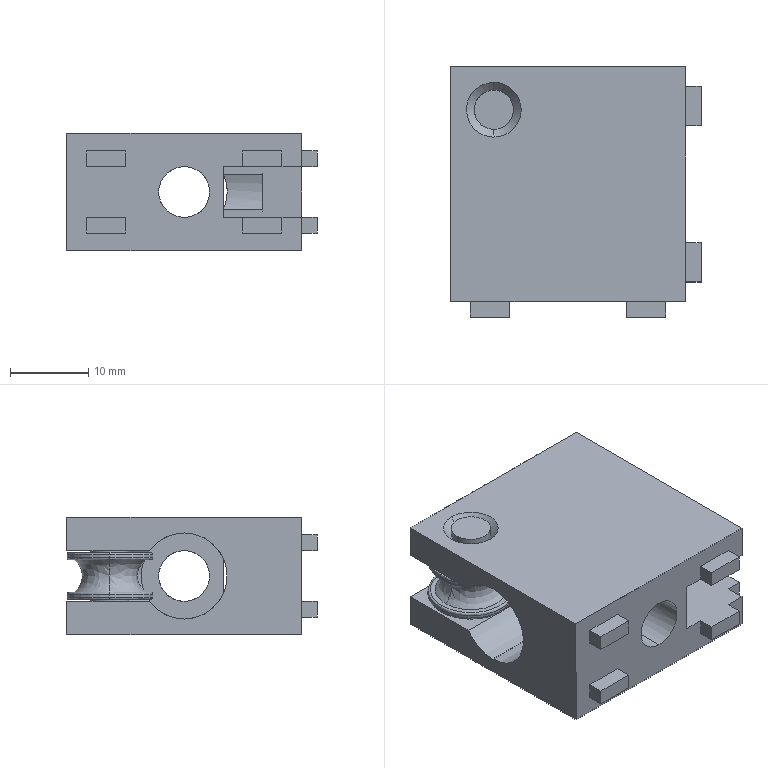Part | SolidWorks | features BaseBody 1 | 1 solid | 100 faces | box 32 x 32 x 15 mm | volume 8367 mm3 | plane 58 | cylinder 28 | spline 10 | cone 4 | commonest cylinder face diameters 11 x16 5 x8 6.5 x4